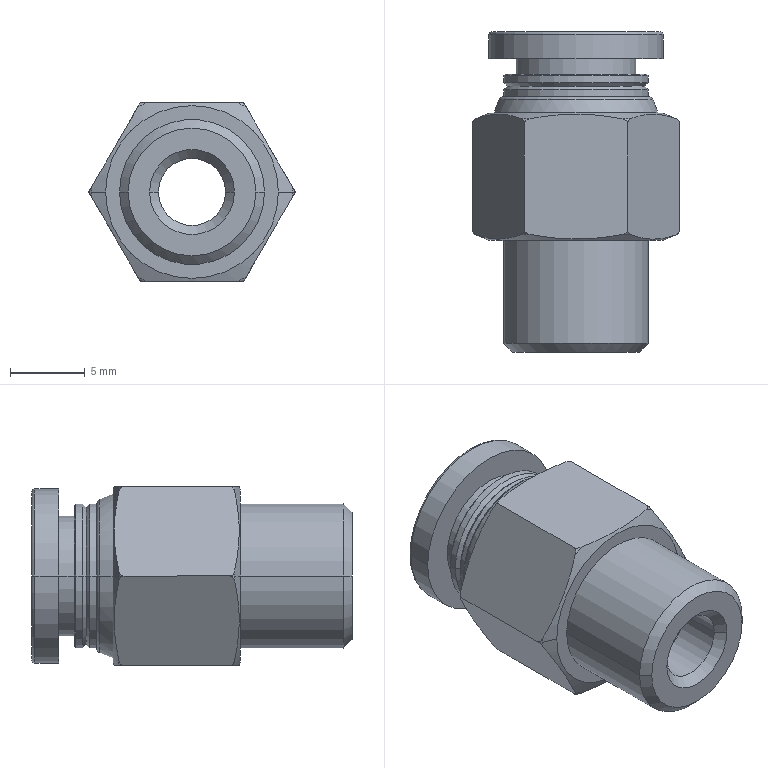Part | SolidWorks | features MBimport 1 | 1 solid | 64 faces | box 13.856 x 21.5 x 12 mm | volume 1497 mm3 | torus 20 | cone 16 | cylinder 14 | plane 14 | commonest cylinder face diameters 9.7 x4 4.5 x2 6 x2 8 x2 9.728 x2 11.7 x2